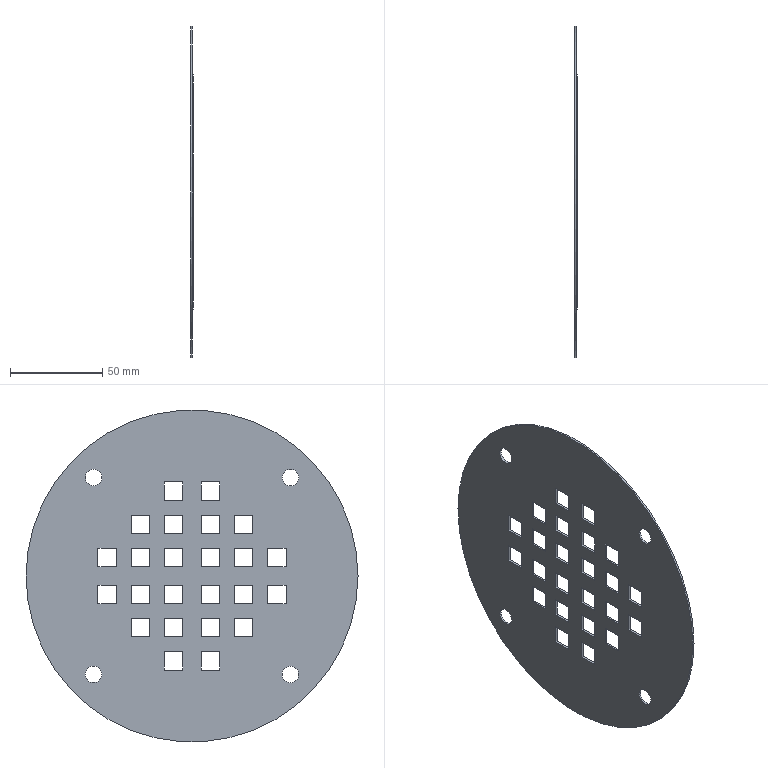Part | STEP file | a-hp_225_37-140_3_0_05 | 1 solid | 107 faces | box 1.5 x 180 x 180 mm | volume 24200 mm3 | plane 100 | cylinder 7 | commonest cylinder face diameters 9 x4 112 x1 127 x1 180 x1